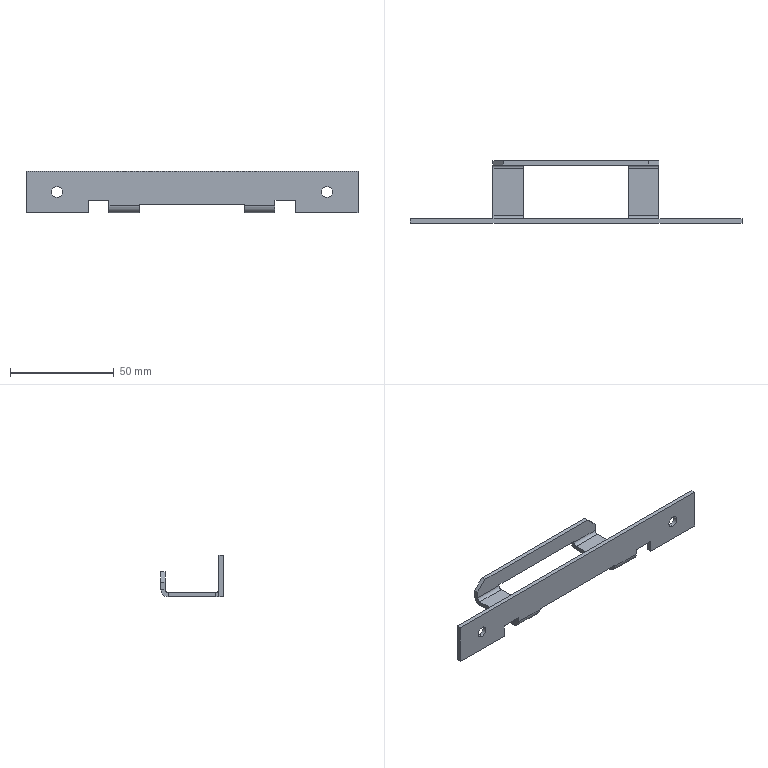Part | STEP file | Slide plate bracket | 1 solid | 54 faces | box 160 x 30 x 20 mm | volume 8510 mm3 | plane 42 | cylinder 12 | commonest cylinder face diameters 3 x4 5.3 x4 7 x4